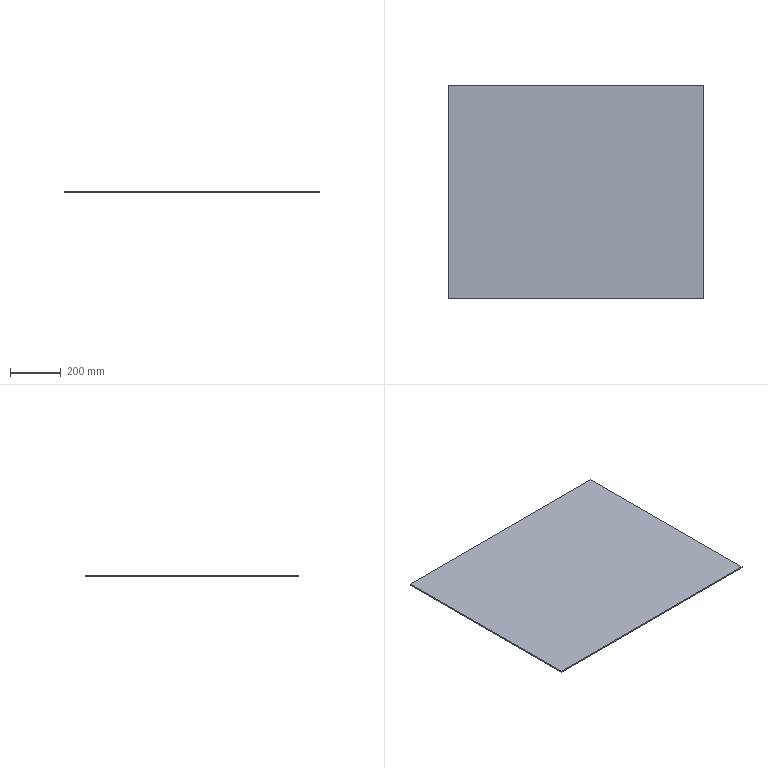Part | SolidWorks | features Extrusion 1, HoleWzd 1 | 1 solid | 6 faces | box 1009 x 842 x 5 mm | volume 4247890 mm3 | plane 6
STEP:
#1=CARTESIAN_POINT('',(504.5,-421.,0.));
#2=VERTEX_POINT('',#1);
#3=CARTESIAN_POINT('',(504.5,421.,0.));
#4=VERTEX_POINT('',#3);
#5=CARTESIAN_POINT('',(504.5,421.,0.));
#6=DIRECTION('',(0.,1.,0.));
#7=VECTOR('',#6,1000.);
#8=LINE('',#5,#7);
#9=EDGE_CURVE('',#2,#4,#8,.T.);
#10=ORIENTED_EDGE('',*,*,#9,.T.);
#11=CARTESIAN_POINT('',(504.5,421.,5.));
#12=VERTEX_POINT('',#11);
#13=CARTESIAN_POINT('',(504.5,421.,5.));
#14=DIRECTION('',(0.,0.,-1.));
#15=VECTOR('',#14,1000.);
#16=LINE('',#13,#15);
#17=EDGE_CURVE('',#12,#4,#16,.T.);
#18=ORIENTED_EDGE('',*,*,#17,.F.);
#19=CARTESIAN_POINT('',(504.5,-421.,5.));
#20=VERTEX_POINT('',#19);
#21=CARTESIAN_POINT('',(504.5,421.,5.));
#22=DIRECTION('',(0.,1.,0.));
#23=VECTOR('',#22,1000.);
#24=LINE('',#21,#23);
#25=EDGE_CURVE('',#20,#12,#24,.T.);
#26=ORIENTED_EDGE('',*,*,#25,.F.);
#27=CARTESIAN_POINT('',(504.5,-421.,5.));
#28=DIRECTION('',(0.,0.,-1.));
#29=VECTOR('',#28,1000.);
#30=LINE('',#27,#29);
#31=EDGE_CURVE('',#20,#2,#30,.T.);
#32=ORIENTED_EDGE('',*,*,#31,.T.);
#33=EDGE_LOOP('',(#10,#18,#26,#32));
#34=FACE_OUTER_BOUND('',#33,.T.);
#35=CARTESIAN_POINT('',(504.5,421.,5.));
#36=DIRECTION('',(-1.,0.,0.));
#37=DIRECTION('',(0.,0.,1.));
#38=AXIS2_PLACEMENT_3D('',#35,#36,#37);
#39=PLANE('',#38);
#40=ADVANCED_FACE('',(#34),#39,.F.);
#41=CARTESIAN_POINT('',(-504.5,421.,0.));
#42=VERTEX_POINT('',#41);
#43=CARTESIAN_POINT('',(-504.5,421.,0.));
#44=DIRECTION('',(-1.,0.,0.));
#45=VECTOR('',#44,1000.);
#46=LINE('',#43,#45);
#47=EDGE_CURVE('',#4,#42,#46,.T.);
#48=ORIENTED_EDGE('',*,*,#47,.T.);
#49=CARTESIAN_POINT('',(-504.5,421.,5.));
#50=VERTEX_POINT('',#49);
#51=CARTESIAN_POINT('',(-504.5,421.,5.));
#52=DIRECTION('',(0.,0.,-1.));
#53=VECTOR('',#52,1000.);
#54=LINE('',#51,#53);
#55=EDGE_CURVE('',#50,#42,#54,.T.);
#56=ORIENTED_EDGE('',*,*,#55,.F.);
#57=CARTESIAN_POINT('',(-504.5,421.,5.));
#58=DIRECTION('',(-1.,0.,0.));
#59=VECTOR('',#58,1000.);
#60=LINE('',#57,#59);
#61=EDGE_CURVE('',#12,#50,#60,.T.);
#62=ORIENTED_EDGE('',*,*,#61,.F.);
#63=ORIENTED_EDGE('',*,*,#17,.T.);
#64=EDGE_LOOP('',(#48,#56,#62,#63));
#65=FACE_OUTER_BOUND('',#64,.T.);
#66=CARTESIAN_POINT('',(-504.5,421.,5.));
#67=DIRECTION('',(0.,-1.,0.));
#68=DIRECTION('',(0.,0.,-1.));
#69=AXIS2_PLACEMENT_3D('',#66,#67,#68);
#70=PLANE('',#69);
#71=ADVANCED_FACE('',(#65),#70,.F.);
#72=CARTESIAN_POINT('',(-504.5,-421.,0.));
#73=VERTEX_POINT('',#72);
#74=CARTESIAN_POINT('',(-504.5,421.,0.));
#75=DIRECTION('',(0.,-1.,0.));
#76=VECTOR('',#75,1000.);
#77=LINE('',#74,#76);
#78=EDGE_CURVE('',#42,#73,#77,.T.);
#79=ORIENTED_EDGE('',*,*,#78,.T.);
#80=CARTESIAN_POINT('',(-504.5,-421.,5.));
#81=VERTEX_POINT('',#80);
#82=CARTESIAN_POINT('',(-504.5,-421.,5.));
#83=DIRECTION('',(0.,0.,-1.));
#84=VECTOR('',#83,1000.);
#85=LINE('',#82,#84);
#86=EDGE_CURVE('',#81,#73,#85,.T.);
#87=ORIENTED_EDGE('',*,*,#86,.F.);
#88=CARTESIAN_POINT('',(-504.5,421.,5.));
#89=DIRECTION('',(0.,-1.,0.));
#90=VECTOR('',#89,1000.);
#91=LINE('',#88,#90);
#92=EDGE_CURVE('',#50,#81,#91,.T.);
#93=ORIENTED_EDGE('',*,*,#92,.F.);
#94=ORIENTED_EDGE('',*,*,#55,.T.);
#95=EDGE_LOOP('',(#79,#87,#93,#94));
#96=FACE_OUTER_BOUND('',#95,.T.);
#97=CARTESIAN_POINT('',(-504.5,421.,5.));
#98=DIRECTION('',(1.,0.,0.));
#99=DIRECTION('',(0.,0.,-1.));
#100=AXIS2_PLACEMENT_3D('',#97,#98,#99);
#101=PLANE('',#100);
#102=ADVANCED_FACE('',(#96),#101,.F.);
#103=CARTESIAN_POINT('',(-504.5,-421.,0.));
#104=DIRECTION('',(1.,0.,0.));
#105=VECTOR('',#104,1000.);
#106=LINE('',#103,#105);
#107=EDGE_CURVE('',#73,#2,#106,.T.);
#108=ORIENTED_EDGE('',*,*,#107,.T.);
#109=ORIENTED_EDGE('',*,*,#31,.F.);
#110=CARTESIAN_POINT('',(-504.5,-421.,5.));
#111=DIRECTION('',(1.,0.,0.));
#112=VECTOR('',#111,1000.);
#113=LINE('',#110,#112);
#114=EDGE_CURVE('',#81,#20,#113,.T.);
#115=ORIENTED_EDGE('',*,*,#114,.F.);
#116=ORIENTED_EDGE('',*,*,#86,.T.);
#117=EDGE_LOOP('',(#108,#109,#115,#116));
#118=FACE_OUTER_BOUND('',#117,.T.);
#119=CARTESIAN_POINT('',(-504.5,-421.,5.));
#120=DIRECTION('',(0.,1.,0.));
#121=DIRECTION('',(0.,0.,1.));
#122=AXIS2_PLACEMENT_3D('',#119,#120,#121);
#123=PLANE('',#122);
#124=ADVANCED_FACE('',(#118),#123,.F.);
#125=ORIENTED_EDGE('',*,*,#25,.T.);
#126=ORIENTED_EDGE('',*,*,#61,.T.);
#127=ORIENTED_EDGE('',*,*,#92,.T.);
#128=ORIENTED_EDGE('',*,*,#114,.T.);
#129=EDGE_LOOP('',(#125,#126,#127,#128));
#130=FACE_OUTER_BOUND('',#129,.T.);
#131=CARTESIAN_POINT('',(0.,0.,5.));
#132=DIRECTION('',(0.,0.,1.));
#133=DIRECTION('',(1.,0.,0.));
#134=AXIS2_PLACEMENT_3D('',#131,#132,#133);
#135=PLANE('',#134);
#136=ADVANCED_FACE('',(#130),#135,.T.);
#137=ORIENTED_EDGE('',*,*,#9,.F.);
#138=ORIENTED_EDGE('',*,*,#107,.F.);
#139=ORIENTED_EDGE('',*,*,#78,.F.);
#140=ORIENTED_EDGE('',*,*,#47,.F.);
#141=EDGE_LOOP('',(#137,#138,#139,#140));
#142=FACE_OUTER_BOUND('',#141,.T.);
#143=CARTESIAN_POINT('',(0.,0.,0.));
#144=DIRECTION('',(0.,0.,1.));
#145=DIRECTION('',(1.,0.,0.));
#146=AXIS2_PLACEMENT_3D('',#143,#144,#145);
#147=PLANE('',#146);
#148=ADVANCED_FACE('',(#142),#147,.F.);
#149=CLOSED_SHELL('',(#40,#71,#102,#124,#136,#148));
#150=MANIFOLD_SOLID_BREP('',#149);
#151=CARTESIAN_POINT('',(0.,0.,0.));
#152=DIRECTION('',(0.,0.,1.));
#153=DIRECTION('',(1.,0.,0.));
#154=AXIS2_PLACEMENT_3D('',#151,#152,#153);
#155=(LENGTH_UNIT()NAMED_UNIT(*)SI_UNIT(.MILLI.,.METRE.));
#156=UNCERTAINTY_MEASURE_WITH_UNIT(LENGTH_MEASURE(0.00001),#155,'','');
#157=(NAMED_UNIT(*)PLANE_ANGLE_UNIT()SI_UNIT($,.RADIAN.));
#158=(NAMED_UNIT(*)SI_UNIT($,.STERADIAN.)SOLID_ANGLE_UNIT());
#159=(GEOMETRIC_REPRESENTATION_CONTEXT(3)GLOBAL_UNCERTAINTY_ASSIGNED_CONTEXT((#156))GLOBAL_UNIT_ASSIGNED_CONTEXT((#155,#157,#158))REPRESENTATION_CONTEXT('',''));
#160=ADVANCED_BREP_SHAPE_REPRESENTATION('',(#150,#154),#159);